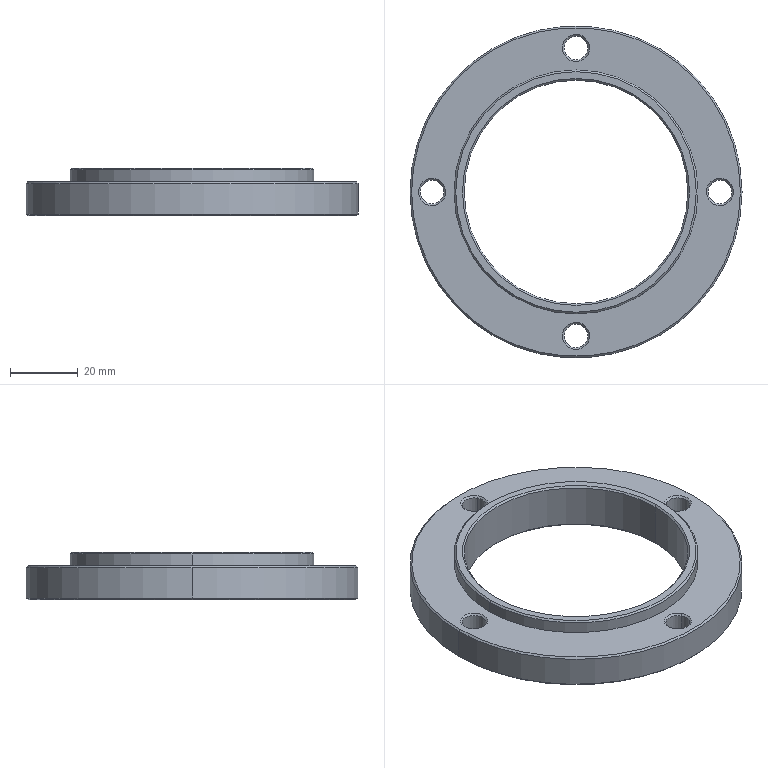Part | STEP file | 20322 | 1 solid | 43 faces | box 98 x 98 x 14 mm | volume 42100 mm3 | cone 26 | cylinder 14 | plane 3 | commonest cylinder face diameters 7 x8 66 x2 72 x2 98 x2
STEP:
#1=CARTESIAN_POINT('',(48.5,0.,10.));
#2=VERTEX_POINT('',#1);
#3=CARTESIAN_POINT('',(49.,0.,9.5));
#4=VERTEX_POINT('',#3);
#5=CARTESIAN_POINT('',(48.75,0.,9.75));
#6=DIRECTION('',(0.7071,0.,-0.7071));
#7=VECTOR('',#6,1.);
#8=LINE('',#5,#7);
#9=EDGE_CURVE('',#2,#4,#8,.T.);
#10=ORIENTED_EDGE('',*,*,#9,.T.);
#11=CARTESIAN_POINT('',(-49.,0.,9.5));
#12=VERTEX_POINT('',#11);
#13=CARTESIAN_POINT('',(0.,0.,9.5));
#14=DIRECTION('',(0.,0.,1.));
#15=AXIS2_PLACEMENT_3D('',#13,#14,$);
#16=CIRCLE('',#15,49.);
#17=EDGE_CURVE('',#4,#12,#16,.T.);
#18=ORIENTED_EDGE('',*,*,#17,.T.);
#19=CARTESIAN_POINT('',(-48.5,0.000000485,10.));
#20=VERTEX_POINT('',#19);
#21=CARTESIAN_POINT('',(-48.75,0.,9.75));
#22=DIRECTION('',(-0.7071,0.,-0.7071));
#23=VECTOR('',#22,1.);
#24=LINE('',#21,#23);
#25=EDGE_CURVE('',#20,#12,#24,.T.);
#26=ORIENTED_EDGE('',*,*,#25,.F.);
#27=CARTESIAN_POINT('',(0.,0.,10.));
#28=DIRECTION('',(0.,0.,1.));
#29=AXIS2_PLACEMENT_3D('',#27,#28,$);
#30=CIRCLE('',#29,48.5);
#31=EDGE_CURVE('',#2,#20,#30,.T.);
#32=ORIENTED_EDGE('',*,*,#31,.F.);
#33=EDGE_LOOP('',(#10,#18,#26,#32));
#34=FACE_OUTER_BOUND('',#33,.T.);
#35=CARTESIAN_POINT('',(0.,0.,58.5));
#36=DIRECTION('',(0.,0.,-1.));
#37=DIRECTION('',(1.,0.,0.));
#38=AXIS2_PLACEMENT_3D('',#35,#36,#37);
#39=CONICAL_SURFACE('',#38,0.,0.7854);
#40=ADVANCED_FACE('',(#34),#39,.T.);
#41=ORIENTED_EDGE('',*,*,#25,.T.);
#42=CARTESIAN_POINT('',(0.,0.,9.5));
#43=DIRECTION('',(0.,0.,1.));
#44=AXIS2_PLACEMENT_3D('',#42,#43,$);
#45=CIRCLE('',#44,49.);
#46=EDGE_CURVE('',#12,#4,#45,.T.);
#47=ORIENTED_EDGE('',*,*,#46,.T.);
#48=ORIENTED_EDGE('',*,*,#9,.F.);
#49=CARTESIAN_POINT('',(0.,0.,10.));
#50=DIRECTION('',(0.,0.,1.));
#51=AXIS2_PLACEMENT_3D('',#49,#50,$);
#52=CIRCLE('',#51,48.5);
#53=EDGE_CURVE('',#20,#2,#52,.T.);
#54=ORIENTED_EDGE('',*,*,#53,.F.);
#55=EDGE_LOOP('',(#41,#47,#48,#54));
#56=FACE_OUTER_BOUND('',#55,.T.);
#57=CARTESIAN_POINT('',(0.,0.,58.5));
#58=DIRECTION('',(0.,0.,-1.));
#59=DIRECTION('',(-1.,0.,0.));
#60=AXIS2_PLACEMENT_3D('',#57,#58,#59);
#61=CONICAL_SURFACE('',#60,0.,0.7854);
#62=ADVANCED_FACE('',(#56),#61,.T.);
#63=CARTESIAN_POINT('',(-49.,0.,0.5));
#64=VERTEX_POINT('',#63);
#65=CARTESIAN_POINT('',(-49.,0.,5.));
#66=DIRECTION('',(0.,0.,1.));
#67=VECTOR('',#66,1.);
#68=LINE('',#65,#67);
#69=EDGE_CURVE('',#64,#12,#68,.T.);
#70=ORIENTED_EDGE('',*,*,#69,.T.);
#71=ORIENTED_EDGE('',*,*,#17,.F.);
#72=CARTESIAN_POINT('',(49.,0.,0.5));
#73=VERTEX_POINT('',#72);
#74=CARTESIAN_POINT('',(49.,0.,5.));
#75=DIRECTION('',(0.,0.,1.));
#76=VECTOR('',#75,1.);
#77=LINE('',#74,#76);
#78=EDGE_CURVE('',#73,#4,#77,.T.);
#79=ORIENTED_EDGE('',*,*,#78,.F.);
#80=CARTESIAN_POINT('',(0.,0.,0.5));
#81=DIRECTION('',(0.,0.,1.));
#82=AXIS2_PLACEMENT_3D('',#80,#81,$);
#83=CIRCLE('',#82,49.);
#84=EDGE_CURVE('',#73,#64,#83,.T.);
#85=ORIENTED_EDGE('',*,*,#84,.T.);
#86=EDGE_LOOP('',(#70,#71,#79,#85));
#87=FACE_OUTER_BOUND('',#86,.T.);
#88=CARTESIAN_POINT('',(0.,0.,5.));
#89=DIRECTION('',(0.,0.,1.));
#90=DIRECTION('',(1.,0.,0.));
#91=AXIS2_PLACEMENT_3D('',#88,#89,#90);
#92=CYLINDRICAL_SURFACE('',#91,49.);
#93=ADVANCED_FACE('',(#87),#92,.T.);
#94=ORIENTED_EDGE('',*,*,#78,.T.);
#95=ORIENTED_EDGE('',*,*,#46,.F.);
#96=ORIENTED_EDGE('',*,*,#69,.F.);
#97=CARTESIAN_POINT('',(0.,0.,0.5));
#98=DIRECTION('',(0.,0.,1.));
#99=AXIS2_PLACEMENT_3D('',#97,#98,$);
#100=CIRCLE('',#99,49.);
#101=EDGE_CURVE('',#64,#73,#100,.T.);
#102=ORIENTED_EDGE('',*,*,#101,.T.);
#103=EDGE_LOOP('',(#94,#95,#96,#102));
#104=FACE_OUTER_BOUND('',#103,.T.);
#105=ADVANCED_FACE('',(#104),#92,.T.);
#106=CARTESIAN_POINT('',(48.5,0.,0.));
#107=VERTEX_POINT('',#106);
#108=CARTESIAN_POINT('',(48.75,0.,0.25));
#109=DIRECTION('',(0.7071,0.,0.7071));
#110=VECTOR('',#109,1.);
#111=LINE('',#108,#110);
#112=EDGE_CURVE('',#73,#107,#111,.F.);
#113=ORIENTED_EDGE('',*,*,#112,.T.);
#114=CARTESIAN_POINT('',(-48.5,0.000000092,0.));
#115=VERTEX_POINT('',#114);
#116=CARTESIAN_POINT('',(0.,0.,0.));
#117=DIRECTION('',(0.,0.,1.));
#118=AXIS2_PLACEMENT_3D('',#116,#117,$);
#119=CIRCLE('',#118,48.5);
#120=EDGE_CURVE('',#107,#115,#119,.T.);
#121=ORIENTED_EDGE('',*,*,#120,.T.);
#122=CARTESIAN_POINT('',(-48.75,0.000000092,0.25));
#123=DIRECTION('',(-0.7071,0.000000001,0.7071));
#124=VECTOR('',#123,1.);
#125=LINE('',#122,#124);
#126=EDGE_CURVE('',#64,#115,#125,.F.);
#127=ORIENTED_EDGE('',*,*,#126,.F.);
#128=ORIENTED_EDGE('',*,*,#84,.F.);
#129=EDGE_LOOP('',(#113,#121,#127,#128));
#130=FACE_OUTER_BOUND('',#129,.T.);
#131=CARTESIAN_POINT('',(0.,0.,-48.5));
#132=DIRECTION('',(0.,0.,1.));
#133=DIRECTION('',(1.,0.,0.));
#134=AXIS2_PLACEMENT_3D('',#131,#132,#133);
#135=CONICAL_SURFACE('',#134,0.,0.7854);
#136=ADVANCED_FACE('',(#130),#135,.T.);
#137=ORIENTED_EDGE('',*,*,#126,.T.);
#138=CARTESIAN_POINT('',(0.,0.,0.));
#139=DIRECTION('',(0.,0.,1.));
#140=AXIS2_PLACEMENT_3D('',#138,#139,$);
#141=CIRCLE('',#140,48.5);
#142=EDGE_CURVE('',#115,#107,#141,.T.);
#143=ORIENTED_EDGE('',*,*,#142,.T.);
#144=ORIENTED_EDGE('',*,*,#112,.F.);
#145=ORIENTED_EDGE('',*,*,#101,.F.);
#146=EDGE_LOOP('',(#137,#143,#144,#145));
#147=FACE_OUTER_BOUND('',#146,.T.);
#148=CARTESIAN_POINT('',(0.,0.,-48.5));
#149=DIRECTION('',(0.,0.,1.));
#150=DIRECTION('',(-0.9454,0.3259,0.));
#151=AXIS2_PLACEMENT_3D('',#148,#149,#150);
#152=CONICAL_SURFACE('',#151,0.,0.7854);
#153=ADVANCED_FACE('',(#147),#152,.T.);
#154=CARTESIAN_POINT('',(-33.5,-0.000000738,0.));
#155=VERTEX_POINT('',#154);
#156=CARTESIAN_POINT('',(-33.,0.,0.5));
#157=VERTEX_POINT('',#156);
#158=CARTESIAN_POINT('',(-33.25,0.,0.25));
#159=DIRECTION('',(-0.7071,0.,-0.7071));
#160=VECTOR('',#159,1.);
#161=LINE('',#158,#160);
#162=EDGE_CURVE('',#155,#157,#161,.F.);
#163=ORIENTED_EDGE('',*,*,#162,.T.);
#164=CARTESIAN_POINT('',(33.,0.,0.5));
#165=VERTEX_POINT('',#164);
#166=CARTESIAN_POINT('',(0.,0.,0.5));
#167=DIRECTION('',(0.,0.,1.));
#168=AXIS2_PLACEMENT_3D('',#166,#167,$);
#169=CIRCLE('',#168,33.);
#170=EDGE_CURVE('',#157,#165,#169,.T.);
#171=ORIENTED_EDGE('',*,*,#170,.T.);
#172=CARTESIAN_POINT('',(33.5,0.,0.));
#173=VERTEX_POINT('',#172);
#174=CARTESIAN_POINT('',(33.25,0.,0.25));
#175=DIRECTION('',(0.7071,0.,-0.7071));
#176=VECTOR('',#175,1.);
#177=LINE('',#174,#176);
#178=EDGE_CURVE('',#173,#165,#177,.F.);
#179=ORIENTED_EDGE('',*,*,#178,.F.);
#180=CARTESIAN_POINT('',(0.,0.,0.));
#181=DIRECTION('',(0.,0.,1.));
#182=AXIS2_PLACEMENT_3D('',#180,#181,$);
#183=CIRCLE('',#182,33.5);
#184=EDGE_CURVE('',#155,#173,#183,.T.);
#185=ORIENTED_EDGE('',*,*,#184,.F.);
#186=EDGE_LOOP('',(#163,#171,#179,#185));
#187=FACE_OUTER_BOUND('',#186,.T.);
#188=CARTESIAN_POINT('',(0.,0.,33.5));
#189=DIRECTION('',(0.,0.,-1.));
#190=DIRECTION('',(-0.8872,0.4614,0.));
#191=AXIS2_PLACEMENT_3D('',#188,#189,#190);
#192=CONICAL_SURFACE('',#191,0.,0.7854);
#193=ADVANCED_FACE('',(#187),#192,.F.);
#194=ORIENTED_EDGE('',*,*,#178,.T.);
#195=CARTESIAN_POINT('',(0.,0.,0.5));
#196=DIRECTION('',(0.,0.,1.));
#197=AXIS2_PLACEMENT_3D('',#195,#196,$);
#198=CIRCLE('',#197,33.);
#199=EDGE_CURVE('',#165,#157,#198,.T.);
#200=ORIENTED_EDGE('',*,*,#199,.T.);
#201=ORIENTED_EDGE('',*,*,#162,.F.);
#202=CARTESIAN_POINT('',(0.,0.,0.));
#203=DIRECTION('',(0.,0.,1.));
#204=AXIS2_PLACEMENT_3D('',#202,#203,$);
#205=CIRCLE('',#204,33.5);
#206=EDGE_CURVE('',#173,#155,#205,.T.);
#207=ORIENTED_EDGE('',*,*,#206,.F.);
#208=EDGE_LOOP('',(#194,#200,#201,#207));
#209=FACE_OUTER_BOUND('',#208,.T.);
#210=CARTESIAN_POINT('',(0.,0.,33.5));
#211=DIRECTION('',(0.,0.,-1.));
#212=DIRECTION('',(1.,0.,0.));
#213=AXIS2_PLACEMENT_3D('',#210,#211,#212);
#214=CONICAL_SURFACE('',#213,0.,0.7854);
#215=ADVANCED_FACE('',(#209),#214,.F.);
#216=ORIENTED_EDGE('',*,*,#170,.F.);
#217=CARTESIAN_POINT('',(-33.,0.,13.5));
#218=VERTEX_POINT('',#217);
#219=CARTESIAN_POINT('',(-33.,0.,5.));
#220=DIRECTION('',(0.,0.,1.));
#221=VECTOR('',#220,1.);
#222=LINE('',#219,#221);
#223=EDGE_CURVE('',#218,#157,#222,.F.);
#224=ORIENTED_EDGE('',*,*,#223,.F.);
#225=CARTESIAN_POINT('',(33.,0.,13.5));
#226=VERTEX_POINT('',#225);
#227=CARTESIAN_POINT('',(0.,0.,13.5));
#228=DIRECTION('',(0.,0.,1.));
#229=AXIS2_PLACEMENT_3D('',#227,#228,$);
#230=CIRCLE('',#229,33.);
#231=EDGE_CURVE('',#218,#226,#230,.T.);
#232=ORIENTED_EDGE('',*,*,#231,.T.);
#233=CARTESIAN_POINT('',(33.,0.,5.));
#234=DIRECTION('',(0.,0.,1.));
#235=VECTOR('',#234,1.);
#236=LINE('',#233,#235);
#237=EDGE_CURVE('',#226,#165,#236,.F.);
#238=ORIENTED_EDGE('',*,*,#237,.T.);
#239=EDGE_LOOP('',(#216,#224,#232,#238));
#240=FACE_OUTER_BOUND('',#239,.T.);
#241=CARTESIAN_POINT('',(0.,0.,5.));
#242=DIRECTION('',(0.,0.,1.));
#243=DIRECTION('',(1.,0.,0.));
#244=AXIS2_PLACEMENT_3D('',#241,#242,#243);
#245=CYLINDRICAL_SURFACE('',#244,33.);
#246=ADVANCED_FACE('',(#240),#245,.F.);
#247=ORIENTED_EDGE('',*,*,#199,.F.);
#248=ORIENTED_EDGE('',*,*,#237,.F.);
#249=CARTESIAN_POINT('',(0.,0.,13.5));
#250=DIRECTION('',(0.,0.,1.));
#251=AXIS2_PLACEMENT_3D('',#249,#250,$);
#252=CIRCLE('',#251,33.);
#253=EDGE_CURVE('',#226,#218,#252,.T.);
#254=ORIENTED_EDGE('',*,*,#253,.T.);
#255=ORIENTED_EDGE('',*,*,#223,.T.);
#256=EDGE_LOOP('',(#247,#248,#254,#255));
#257=FACE_OUTER_BOUND('',#256,.T.);
#258=ADVANCED_FACE('',(#257),#245,.F.);
#259=CARTESIAN_POINT('',(-33.5,0.000000544,14.));
#260=VERTEX_POINT('',#259);
#261=CARTESIAN_POINT('',(-33.25,0.,13.75));
#262=DIRECTION('',(-0.7071,0.,0.7071));
#263=VECTOR('',#262,1.);
#264=LINE('',#261,#263);
#265=EDGE_CURVE('',#218,#260,#264,.T.);
#266=ORIENTED_EDGE('',*,*,#265,.T.);
#267=CARTESIAN_POINT('',(33.5,0.,14.));
#268=VERTEX_POINT('',#267);
#269=CARTESIAN_POINT('',(0.,0.,14.));
#270=DIRECTION('',(0.,0.,1.));
#271=AXIS2_PLACEMENT_3D('',#269,#270,$);
#272=CIRCLE('',#271,33.5);
#273=EDGE_CURVE('',#260,#268,#272,.T.);
#274=ORIENTED_EDGE('',*,*,#273,.T.);
#275=CARTESIAN_POINT('',(33.25,0.,13.75));
#276=DIRECTION('',(0.7071,0.,0.7071));
#277=VECTOR('',#276,1.);
#278=LINE('',#275,#277);
#279=EDGE_CURVE('',#226,#268,#278,.T.);
#280=ORIENTED_EDGE('',*,*,#279,.F.);
#281=ORIENTED_EDGE('',*,*,#231,.F.);
#282=EDGE_LOOP('',(#266,#274,#280,#281));
#283=FACE_OUTER_BOUND('',#282,.T.);
#284=CARTESIAN_POINT('',(0.,0.,-19.5));
#285=DIRECTION('',(0.,0.,1.));
#286=DIRECTION('',(-0.9714,0.2374,0.));
#287=AXIS2_PLACEMENT_3D('',#284,#285,#286);
#288=CONICAL_SURFACE('',#287,0.,0.7854);
#289=ADVANCED_FACE('',(#283),#288,.F.);
#290=ORIENTED_EDGE('',*,*,#279,.T.);
#291=CARTESIAN_POINT('',(0.,0.,14.));
#292=DIRECTION('',(0.,0.,1.));
#293=AXIS2_PLACEMENT_3D('',#291,#292,$);
#294=CIRCLE('',#293,33.5);
#295=EDGE_CURVE('',#268,#260,#294,.T.);
#296=ORIENTED_EDGE('',*,*,#295,.T.);
#297=ORIENTED_EDGE('',*,*,#265,.F.);
#298=ORIENTED_EDGE('',*,*,#253,.F.);
#299=EDGE_LOOP('',(#290,#296,#297,#298));
#300=FACE_OUTER_BOUND('',#299,.T.);
#301=CARTESIAN_POINT('',(0.,0.,-19.5));
#302=DIRECTION('',(0.,0.,1.));
#303=DIRECTION('',(1.,0.,0.));
#304=AXIS2_PLACEMENT_3D('',#301,#302,#303);
#305=CONICAL_SURFACE('',#304,0.,0.7854);
#306=ADVANCED_FACE('',(#300),#305,.F.);
#307=CARTESIAN_POINT('',(35.5,0.,14.));
#308=VERTEX_POINT('',#307);
#309=CARTESIAN_POINT('',(-35.5,0.000000674,14.));
#310=VERTEX_POINT('',#309);
#311=CARTESIAN_POINT('',(0.,0.,14.));
#312=DIRECTION('',(0.,0.,1.));
#313=AXIS2_PLACEMENT_3D('',#311,#312,$);
#314=CIRCLE('',#313,35.5);
#315=EDGE_CURVE('',#308,#310,#314,.T.);
#316=ORIENTED_EDGE('',*,*,#315,.T.);
#317=CARTESIAN_POINT('',(0.,0.,14.));
#318=DIRECTION('',(0.,0.,1.));
#319=AXIS2_PLACEMENT_3D('',#317,#318,$);
#320=CIRCLE('',#319,35.5);
#321=EDGE_CURVE('',#310,#308,#320,.T.);
#322=ORIENTED_EDGE('',*,*,#321,.T.);
#323=EDGE_LOOP('',(#316,#322));
#324=FACE_OUTER_BOUND('',#323,.T.);
#325=ORIENTED_EDGE('',*,*,#273,.F.);
#326=ORIENTED_EDGE('',*,*,#295,.F.);
#327=EDGE_LOOP('',(#325,#326));
#328=FACE_BOUND('',#327,.T.);
#329=CARTESIAN_POINT('',(0.,0.,14.));
#330=DIRECTION('',(0.,0.,1.));
#331=DIRECTION('',(1.,0.,0.));
#332=AXIS2_PLACEMENT_3D('',#329,#330,#331);
#333=PLANE('',#332);
#334=ADVANCED_FACE('',(#324,#328),#333,.T.);
#335=CARTESIAN_POINT('',(36.,0.,13.5));
#336=VERTEX_POINT('',#335);
#337=CARTESIAN_POINT('',(35.75,0.,13.75));
#338=DIRECTION('',(0.7071,0.,-0.7071));
#339=VECTOR('',#338,1.);
#340=LINE('',#337,#339);
#341=EDGE_CURVE('',#308,#336,#340,.T.);
#342=ORIENTED_EDGE('',*,*,#341,.T.);
#343=CARTESIAN_POINT('',(-36.,0.,13.5));
#344=VERTEX_POINT('',#343);
#345=CARTESIAN_POINT('',(0.,0.,13.5));
#346=DIRECTION('',(0.,0.,1.));
#347=AXIS2_PLACEMENT_3D('',#345,#346,$);
#348=CIRCLE('',#347,36.);
#349=EDGE_CURVE('',#336,#344,#348,.T.);
#350=ORIENTED_EDGE('',*,*,#349,.T.);
#351=CARTESIAN_POINT('',(-35.75,0.,13.75));
#352=DIRECTION('',(-0.7071,0.,-0.7071));
#353=VECTOR('',#352,1.);
#354=LINE('',#351,#353);
#355=EDGE_CURVE('',#310,#344,#354,.T.);
#356=ORIENTED_EDGE('',*,*,#355,.F.);
#357=ORIENTED_EDGE('',*,*,#315,.F.);
#358=EDGE_LOOP('',(#342,#350,#356,#357));
#359=FACE_OUTER_BOUND('',#358,.T.);
#360=CARTESIAN_POINT('',(0.,0.,49.5));
#361=DIRECTION('',(0.,0.,-1.));
#362=DIRECTION('',(1.,0.,0.));
#363=AXIS2_PLACEMENT_3D('',#360,#361,#362);
#364=CONICAL_SURFACE('',#363,0.,0.7854);
#365=ADVANCED_FACE('',(#359),#364,.T.);
#366=ORIENTED_EDGE('',*,*,#355,.T.);
#367=CARTESIAN_POINT('',(0.,0.,13.5));
#368=DIRECTION('',(0.,0.,1.));
#369=AXIS2_PLACEMENT_3D('',#367,#368,$);
#370=CIRCLE('',#369,36.);
#371=EDGE_CURVE('',#344,#336,#370,.T.);
#372=ORIENTED_EDGE('',*,*,#371,.T.);
#373=ORIENTED_EDGE('',*,*,#341,.F.);
#374=ORIENTED_EDGE('',*,*,#321,.F.);
#375=EDGE_LOOP('',(#366,#372,#373,#374));
#376=FACE_OUTER_BOUND('',#375,.T.);
#377=CARTESIAN_POINT('',(0.,0.,49.5));
#378=DIRECTION('',(0.,0.,-1.));
#379=DIRECTION('',(-0.9522,0.3055,0.));
#380=AXIS2_PLACEMENT_3D('',#377,#378,#379);
#381=CONICAL_SURFACE('',#380,0.,0.7854);
#382=ADVANCED_FACE('',(#376),#381,.T.);
#383=CARTESIAN_POINT('',(-36.,0.,10.));
#384=VERTEX_POINT('',#383);
#385=CARTESIAN_POINT('',(-36.,0.,12.));
#386=DIRECTION('',(0.,0.,1.));
#387=VECTOR('',#386,1.);
#388=LINE('',#385,#387);
#389=EDGE_CURVE('',#384,#344,#388,.T.);
#390=ORIENTED_EDGE('',*,*,#389,.F.);
#391=CARTESIAN_POINT('',(36.,0.,10.));
#392=VERTEX_POINT('',#391);
#393=CARTESIAN_POINT('',(0.,0.,10.));
#394=DIRECTION('',(0.,0.,1.));
#395=AXIS2_PLACEMENT_3D('',#393,#394,$);
#396=CIRCLE('',#395,36.);
#397=EDGE_CURVE('',#384,#392,#396,.T.);
#398=ORIENTED_EDGE('',*,*,#397,.T.);
#399=CARTESIAN_POINT('',(36.,0.,12.));
#400=DIRECTION('',(0.,0.,1.));
#401=VECTOR('',#400,1.);
#402=LINE('',#399,#401);
#403=EDGE_CURVE('',#392,#336,#402,.T.);
#404=ORIENTED_EDGE('',*,*,#403,.T.);
#405=ORIENTED_EDGE('',*,*,#371,.F.);
#406=EDGE_LOOP('',(#390,#398,#404,#405));
#407=FACE_OUTER_BOUND('',#406,.T.);
#408=CARTESIAN_POINT('',(0.,0.,12.));
#409=DIRECTION('',(0.,0.,1.));
#410=DIRECTION('',(1.,0.,0.));
#411=AXIS2_PLACEMENT_3D('',#408,#409,#410);
#412=CYLINDRICAL_SURFACE('',#411,36.);
#413=ADVANCED_FACE('',(#407),#412,.T.);
#414=ORIENTED_EDGE('',*,*,#403,.F.);
#415=CARTESIAN_POINT('',(0.,0.,10.));
#416=DIRECTION('',(0.,0.,1.));
#417=AXIS2_PLACEMENT_3D('',#415,#416,$);
#418=CIRCLE('',#417,36.);
#419=EDGE_CURVE('',#392,#384,#418,.T.);
#420=ORIENTED_EDGE('',*,*,#419,.T.);
#421=ORIENTED_EDGE('',*,*,#389,.T.);
#422=ORIENTED_EDGE('',*,*,#349,.F.);
#423=EDGE_LOOP('',(#414,#420,#421,#422));
#424=FACE_OUTER_BOUND('',#423,.T.);
#425=ADVANCED_FACE('',(#424),#412,.T.);
#426=CARTESIAN_POINT('',(40.582,3.51,0.));
#427=VERTEX_POINT('',#426);
#428=CARTESIAN_POINT('',(40.822,3.072,0.5));
#429=VERTEX_POINT('',#428);
#430=CARTESIAN_POINT('',(40.702,3.291,0.25));
#431=DIRECTION('',(-0.339,0.6205,-0.7071));
#432=VECTOR('',#431,1.);
#433=LINE('',#430,#432);
#434=EDGE_CURVE('',#427,#429,#433,.F.);
#435=ORIENTED_EDGE('',*,*,#434,.T.);
#436=CARTESIAN_POINT('',(44.178,-3.072,0.5));
#437=VERTEX_POINT('',#436);
#438=CARTESIAN_POINT('',(42.5,0.,0.5));
#439=DIRECTION('',(0.,0.,1.));
#440=AXIS2_PLACEMENT_3D('',#438,#439,$);
#441=CIRCLE('',#440,3.5);
#442=EDGE_CURVE('',#429,#437,#441,.T.);
#443=ORIENTED_EDGE('',*,*,#442,.T.);
#444=CARTESIAN_POINT('',(44.418,-3.51,0.));
#445=VERTEX_POINT('',#444);
#446=CARTESIAN_POINT('',(44.298,-3.291,0.25));
#447=DIRECTION('',(0.339,-0.6205,-0.7071));
#448=VECTOR('',#447,1.);
#449=LINE('',#446,#448);
#450=EDGE_CURVE('',#445,#437,#449,.F.);
#451=ORIENTED_EDGE('',*,*,#450,.F.);
#452=CARTESIAN_POINT('',(42.5,0.,0.));
#453=DIRECTION('',(0.,0.,1.));
#454=AXIS2_PLACEMENT_3D('',#452,#453,$);
#455=CIRCLE('',#454,4.);
#456=EDGE_CURVE('',#427,#445,#455,.T.);
#457=ORIENTED_EDGE('',*,*,#456,.F.);
#458=EDGE_LOOP('',(#435,#443,#451,#457));
#459=FACE_OUTER_BOUND('',#458,.T.);
#460=CARTESIAN_POINT('',(42.5,0.,4.));
#461=DIRECTION('',(0.,0.,-1.));
#462=DIRECTION('',(-0.4794,0.8776,0.));
#463=AXIS2_PLACEMENT_3D('',#460,#461,#462);
#464=CONICAL_SURFACE('',#463,0.,0.7854);
#465=ADVANCED_FACE('',(#459),#464,.F.);
#466=ORIENTED_EDGE('',*,*,#450,.T.);
#467=CARTESIAN_POINT('',(42.5,0.,0.5));
#468=DIRECTION('',(0.,0.,1.));
#469=AXIS2_PLACEMENT_3D('',#467,#468,$);
#470=CIRCLE('',#469,3.5);
#471=EDGE_CURVE('',#437,#429,#470,.T.);
#472=ORIENTED_EDGE('',*,*,#471,.T.);
#473=ORIENTED_EDGE('',*,*,#434,.F.);
#474=CARTESIAN_POINT('',(42.5,0.,0.));
#475=DIRECTION('',(0.,0.,1.));
#476=AXIS2_PLACEMENT_3D('',#474,#475,$);
#477=CIRCLE('',#476,4.);
#478=EDGE_CURVE('',#445,#427,#477,.T.);
#479=ORIENTED_EDGE('',*,*,#478,.F.);
#480=EDGE_LOOP('',(#466,#472,#473,#479));
#481=FACE_OUTER_BOUND('',#480,.T.);
#482=CARTESIAN_POINT('',(42.5,0.,4.));
#483=DIRECTION('',(0.,0.,-1.));
#484=DIRECTION('',(0.4794,-0.8776,0.));
#485=AXIS2_PLACEMENT_3D('',#482,#483,#484);
#486=CONICAL_SURFACE('',#485,0.,0.7854);
#487=ADVANCED_FACE('',(#481),#486,.F.);
#488=CARTESIAN_POINT('',(40.822,3.072,9.5));
#489=VERTEX_POINT('',#488);
#490=CARTESIAN_POINT('',(44.178,-3.072,9.5));
#491=VERTEX_POINT('',#490);
#492=CARTESIAN_POINT('',(42.5,0.,9.5));
#493=DIRECTION('',(0.,0.,1.));
#494=AXIS2_PLACEMENT_3D('',#492,#493,$);
#495=CIRCLE('',#494,3.5);
#496=EDGE_CURVE('',#489,#491,#495,.T.);
#497=ORIENTED_EDGE('',*,*,#496,.T.);
#498=CARTESIAN_POINT('',(44.178,-3.072,4.845));
#499=DIRECTION('',(0.,0.,1.));
#500=VECTOR('',#499,1.);
#501=LINE('',#498,#500);
#502=EDGE_CURVE('',#491,#437,#501,.F.);
#503=ORIENTED_EDGE('',*,*,#502,.T.);
#504=ORIENTED_EDGE('',*,*,#442,.F.);
#505=CARTESIAN_POINT('',(40.822,3.072,4.845));
#506=DIRECTION('',(0.,0.,1.));
#507=VECTOR('',#506,1.);
#508=LINE('',#505,#507);
#509=EDGE_CURVE('',#489,#429,#508,.F.);
#510=ORIENTED_EDGE('',*,*,#509,.F.);
#511=EDGE_LOOP('',(#497,#503,#504,#510));
#512=FACE_OUTER_BOUND('',#511,.T.);
#513=CARTESIAN_POINT('',(42.5,0.,0.1));
#514=DIRECTION('',(0.,0.,1.));
#515=DIRECTION('',(-0.4794,0.8776,0.));
#516=AXIS2_PLACEMENT_3D('',#513,#514,#515);
#517=CYLINDRICAL_SURFACE('',#516,3.5);
#518=ADVANCED_FACE('',(#512),#517,.F.);
#519=CARTESIAN_POINT('',(42.5,0.,9.5));
#520=DIRECTION('',(0.,0.,1.));
#521=AXIS2_PLACEMENT_3D('',#519,#520,$);
#522=CIRCLE('',#521,3.5);
#523=EDGE_CURVE('',#491,#489,#522,.T.);
#524=ORIENTED_EDGE('',*,*,#523,.T.);
#525=ORIENTED_EDGE('',*,*,#509,.T.);
#526=ORIENTED_EDGE('',*,*,#471,.F.);
#527=ORIENTED_EDGE('',*,*,#502,.F.);
#528=EDGE_LOOP('',(#524,#525,#526,#527));
#529=FACE_OUTER_BOUND('',#528,.T.);
#530=ADVANCED_FACE('',(#529),#517,.F.);
#531=CARTESIAN_POINT('',(40.582,3.51,10.));
#532=VERTEX_POINT('',#531);
#533=CARTESIAN_POINT('',(40.702,3.291,9.75));
#534=DIRECTION('',(-0.339,0.6205,0.7071));
#535=VECTOR('',#534,1.);
#536=LINE('',#533,#535);
#537=EDGE_CURVE('',#489,#532,#536,.T.);
#538=ORIENTED_EDGE('',*,*,#537,.T.);
#539=CARTESIAN_POINT('',(44.418,-3.51,10.));
#540=VERTEX_POINT('',#539);
#541=CARTESIAN_POINT('',(42.5,0.,10.));
#542=DIRECTION('',(0.,0.,1.));
#543=AXIS2_PLACEMENT_3D('',#541,#542,$);
#544=CIRCLE('',#543,4.);
#545=EDGE_CURVE('',#532,#540,#544,.T.);
#546=ORIENTED_EDGE('',*,*,#545,.T.);
#547=CARTESIAN_POINT('',(44.298,-3.291,9.75));
#548=DIRECTION('',(0.339,-0.6205,0.7071));
#549=VECTOR('',#548,1.);
#550=LINE('',#547,#549);
#551=EDGE_CURVE('',#491,#540,#550,.T.);
#552=ORIENTED_EDGE('',*,*,#551,.F.);
#553=ORIENTED_EDGE('',*,*,#496,.F.);
#554=EDGE_LOOP('',(#538,#546,#552,#553));
#555=FACE_OUTER_BOUND('',#554,.T.);
#556=CARTESIAN_POINT('',(42.5,0.,6.));
#557=DIRECTION('',(0.,0.,1.));
#558=DIRECTION('',(-0.4794,0.8776,0.));
#559=AXIS2_PLACEMENT_3D('',#556,#557,#558);
#560=CONICAL_SURFACE('',#559,0.,0.7854);
#561=ADVANCED_FACE('',(#555),#560,.F.);
#562=ORIENTED_EDGE('',*,*,#551,.T.);
#563=CARTESIAN_POINT('',(42.5,0.,10.));
#564=DIRECTION('',(0.,0.,1.));
#565=AXIS2_PLACEMENT_3D('',#563,#564,$);
#566=CIRCLE('',#565,4.);
#567=EDGE_CURVE('',#540,#532,#566,.T.);
#568=ORIENTED_EDGE('',*,*,#567,.T.);
#569=ORIENTED_EDGE('',*,*,#537,.F.);
#570=ORIENTED_EDGE('',*,*,#523,.F.);
#571=EDGE_LOOP('',(#562,#568,#569,#570));
#572=FACE_OUTER_BOUND('',#571,.T.);
#573=CARTESIAN_POINT('',(42.5,0.,6.));
#574=DIRECTION('',(0.,0.,1.));
#575=DIRECTION('',(-0.128,-0.9918,0.));
#576=AXIS2_PLACEMENT_3D('',#573,#574,#575);
#577=CONICAL_SURFACE('',#576,0.,0.7854);
#578=ADVANCED_FACE('',(#572),#577,.F.);
#579=CARTESIAN_POINT('',(3.51,-40.582,0.));
#580=VERTEX_POINT('',#579);
#581=CARTESIAN_POINT('',(3.072,-40.822,0.5));
#582=VERTEX_POINT('',#581);
#583=CARTESIAN_POINT('',(3.291,-40.702,0.25));
#584=DIRECTION('',(0.6205,0.339,-0.7071));
#585=VECTOR('',#584,1.);
#586=LINE('',#583,#585);
#587=EDGE_CURVE('',#580,#582,#586,.F.);
#588=ORIENTED_EDGE('',*,*,#587,.T.);
#589=CARTESIAN_POINT('',(-3.072,-44.178,0.5));
#590=VERTEX_POINT('',#589);
#591=CARTESIAN_POINT('',(0.,-42.5,0.5));
#592=DIRECTION('',(0.,0.,1.));
#593=AXIS2_PLACEMENT_3D('',#591,#592,$);
#594=CIRCLE('',#593,3.5);
#595=EDGE_CURVE('',#582,#590,#594,.T.);
#596=ORIENTED_EDGE('',*,*,#595,.T.);
#597=CARTESIAN_POINT('',(-3.51,-44.418,0.));
#598=VERTEX_POINT('',#597);
#599=CARTESIAN_POINT('',(-3.291,-44.298,0.25));
#600=DIRECTION('',(-0.6205,-0.339,-0.7071));
#601=VECTOR('',#600,1.);
#602=LINE('',#599,#601);
#603=EDGE_CURVE('',#598,#590,#602,.F.);
#604=ORIENTED_EDGE('',*,*,#603,.F.);
#605=CARTESIAN_POINT('',(0.,-42.5,0.));
#606=DIRECTION('',(0.,0.,1.));
#607=AXIS2_PLACEMENT_3D('',#605,#606,$);
#608=CIRCLE('',#607,4.);
#609=EDGE_CURVE('',#580,#598,#608,.T.);
#610=ORIENTED_EDGE('',*,*,#609,.F.);
#611=EDGE_LOOP('',(#588,#596,#604,#610));
#612=FACE_OUTER_BOUND('',#611,.T.);
#613=CARTESIAN_POINT('',(0.,-42.5,4.));
#614=DIRECTION('',(0.,0.,-1.));
#615=DIRECTION('',(0.8776,0.4794,0.));
#616=AXIS2_PLACEMENT_3D('',#613,#614,#615);
#617=CONICAL_SURFACE('',#616,0.,0.7854);
#618=ADVANCED_FACE('',(#612),#617,.F.);
#619=ORIENTED_EDGE('',*,*,#603,.T.);
#620=CARTESIAN_POINT('',(0.,-42.5,0.5));
#621=DIRECTION('',(0.,0.,1.));
#622=AXIS2_PLACEMENT_3D('',#620,#621,$);
#623=CIRCLE('',#622,3.5);
#624=EDGE_CURVE('',#590,#582,#623,.T.);
#625=ORIENTED_EDGE('',*,*,#624,.T.);
#626=ORIENTED_EDGE('',*,*,#587,.F.);
#627=CARTESIAN_POINT('',(0.,-42.5,0.));
#628=DIRECTION('',(0.,0.,1.));
#629=AXIS2_PLACEMENT_3D('',#627,#628,$);
#630=CIRCLE('',#629,4.);
#631=EDGE_CURVE('',#598,#580,#630,.T.);
#632=ORIENTED_EDGE('',*,*,#631,.F.);
#633=EDGE_LOOP('',(#619,#625,#626,#632));
#634=FACE_OUTER_BOUND('',#633,.T.);
#635=CARTESIAN_POINT('',(0.,-42.5,4.));
#636=DIRECTION('',(0.,0.,-1.));
#637=DIRECTION('',(-0.9995,-0.03244,0.));
#638=AXIS2_PLACEMENT_3D('',#635,#636,#637);
#639=CONICAL_SURFACE('',#638,0.,0.7854);
#640=ADVANCED_FACE('',(#634),#639,.F.);
#641=CARTESIAN_POINT('',(-3.072,-44.178,9.5));
#642=VERTEX_POINT('',#641);
#643=CARTESIAN_POINT('',(3.072,-40.822,9.5));
#644=VERTEX_POINT('',#643);
#645=CARTESIAN_POINT('',(0.,-42.5,9.5));
#646=DIRECTION('',(0.,0.,1.));
#647=AXIS2_PLACEMENT_3D('',#645,#646,$);
#648=CIRCLE('',#647,3.5);
#649=EDGE_CURVE('',#642,#644,#648,.T.);
#650=ORIENTED_EDGE('',*,*,#649,.T.);
#651=CARTESIAN_POINT('',(3.072,-40.822,4.845));
#652=DIRECTION('',(0.,0.,1.));
#653=VECTOR('',#652,1.);
#654=LINE('',#651,#653);
#655=EDGE_CURVE('',#644,#582,#654,.F.);
#656=ORIENTED_EDGE('',*,*,#655,.T.);
#657=ORIENTED_EDGE('',*,*,#624,.F.);
#658=CARTESIAN_POINT('',(-3.072,-44.178,4.845));
#659=DIRECTION('',(0.,0.,1.));
#660=VECTOR('',#659,1.);
#661=LINE('',#658,#660);
#662=EDGE_CURVE('',#642,#590,#661,.F.);
#663=ORIENTED_EDGE('',*,*,#662,.F.);
#664=EDGE_LOOP('',(#650,#656,#657,#663));
#665=FACE_OUTER_BOUND('',#664,.T.);
#666=CARTESIAN_POINT('',(0.,-42.5,0.1));
#667=DIRECTION('',(0.,0.,1.));
#668=DIRECTION('',(0.8776,0.4794,0.));
#669=AXIS2_PLACEMENT_3D('',#666,#667,#668);
#670=CYLINDRICAL_SURFACE('',#669,3.5);
#671=ADVANCED_FACE('',(#665),#670,.F.);
#672=CARTESIAN_POINT('',(0.,-42.5,9.5));
#673=DIRECTION('',(0.,0.,1.));
#674=AXIS2_PLACEMENT_3D('',#672,#673,$);
#675=CIRCLE('',#674,3.5);
#676=EDGE_CURVE('',#644,#642,#675,.T.);
#677=ORIENTED_EDGE('',*,*,#676,.T.);
#678=ORIENTED_EDGE('',*,*,#662,.T.);
#679=ORIENTED_EDGE('',*,*,#595,.F.);
#680=ORIENTED_EDGE('',*,*,#655,.F.);
#681=EDGE_LOOP('',(#677,#678,#679,#680));
#682=FACE_OUTER_BOUND('',#681,.T.);
#683=ADVANCED_FACE('',(#682),#670,.F.);
#684=CARTESIAN_POINT('',(3.51,-40.582,10.));
#685=VERTEX_POINT('',#684);
#686=CARTESIAN_POINT('',(3.291,-40.702,9.75));
#687=DIRECTION('',(0.6205,0.339,0.7071));
#688=VECTOR('',#687,1.);
#689=LINE('',#686,#688);
#690=EDGE_CURVE('',#644,#685,#689,.T.);
#691=ORIENTED_EDGE('',*,*,#690,.T.);
#692=CARTESIAN_POINT('',(-3.51,-44.418,10.));
#693=VERTEX_POINT('',#692);
#694=CARTESIAN_POINT('',(0.,-42.5,10.));
#695=DIRECTION('',(0.,0.,1.));
#696=AXIS2_PLACEMENT_3D('',#694,#695,$);
#697=CIRCLE('',#696,4.);
#698=EDGE_CURVE('',#685,#693,#697,.T.);
#699=ORIENTED_EDGE('',*,*,#698,.T.);
#700=CARTESIAN_POINT('',(-3.291,-44.298,9.75));
#701=DIRECTION('',(-0.6205,-0.339,0.7071));
#702=VECTOR('',#701,1.);
#703=LINE('',#700,#702);
#704=EDGE_CURVE('',#642,#693,#703,.T.);
#705=ORIENTED_EDGE('',*,*,#704,.F.);
#706=ORIENTED_EDGE('',*,*,#676,.F.);
#707=EDGE_LOOP('',(#691,#699,#705,#706));
#708=FACE_OUTER_BOUND('',#707,.T.);
#709=CARTESIAN_POINT('',(0.,-42.5,6.));
#710=DIRECTION('',(0.,0.,1.));
#711=DIRECTION('',(0.8776,0.4794,0.));
#712=AXIS2_PLACEMENT_3D('',#709,#710,#711);
#713=CONICAL_SURFACE('',#712,0.,0.7854);
#714=ADVANCED_FACE('',(#708),#713,.F.);
#715=ORIENTED_EDGE('',*,*,#704,.T.);
#716=CARTESIAN_POINT('',(0.,-42.5,10.));
#717=DIRECTION('',(0.,0.,1.));
#718=AXIS2_PLACEMENT_3D('',#716,#717,$);
#719=CIRCLE('',#718,4.);
#720=EDGE_CURVE('',#693,#685,#719,.T.);
#721=ORIENTED_EDGE('',*,*,#720,.T.);
#722=ORIENTED_EDGE('',*,*,#690,.F.);
#723=ORIENTED_EDGE('',*,*,#649,.F.);
#724=EDGE_LOOP('',(#715,#721,#722,#723));
#725=FACE_OUTER_BOUND('',#724,.T.);
#726=CARTESIAN_POINT('',(0.,-42.5,6.));
#727=DIRECTION('',(0.,0.,1.));
#728=DIRECTION('',(-0.9918,0.128,0.));
#729=AXIS2_PLACEMENT_3D('',#726,#727,#728);
#730=CONICAL_SURFACE('',#729,0.,0.7854);
#731=ADVANCED_FACE('',(#725),#730,.F.);
#732=CARTESIAN_POINT('',(-44.418,3.51,0.));
#733=VERTEX_POINT('',#732);
#734=CARTESIAN_POINT('',(-44.178,3.072,0.5));
#735=VERTEX_POINT('',#734);
#736=CARTESIAN_POINT('',(-44.298,3.291,0.25));
#737=DIRECTION('',(-0.339,0.6205,-0.7071));
#738=VECTOR('',#737,1.);
#739=LINE('',#736,#738);
#740=EDGE_CURVE('',#733,#735,#739,.F.);
#741=ORIENTED_EDGE('',*,*,#740,.T.);
#742=CARTESIAN_POINT('',(-40.822,-3.072,0.5));
#743=VERTEX_POINT('',#742);
#744=CARTESIAN_POINT('',(-42.5,0.,0.5));
#745=DIRECTION('',(0.,0.,1.));
#746=AXIS2_PLACEMENT_3D('',#744,#745,$);
#747=CIRCLE('',#746,3.5);
#748=EDGE_CURVE('',#735,#743,#747,.T.);
#749=ORIENTED_EDGE('',*,*,#748,.T.);
#750=CARTESIAN_POINT('',(-40.582,-3.51,0.));
#751=VERTEX_POINT('',#750);
#752=CARTESIAN_POINT('',(-40.702,-3.291,0.25));
#753=DIRECTION('',(0.339,-0.6205,-0.7071));
#754=VECTOR('',#753,1.);
#755=LINE('',#752,#754);
#756=EDGE_CURVE('',#751,#743,#755,.F.);
#757=ORIENTED_EDGE('',*,*,#756,.F.);
#758=CARTESIAN_POINT('',(-42.5,0.,0.));
#759=DIRECTION('',(0.,0.,1.));
#760=AXIS2_PLACEMENT_3D('',#758,#759,$);
#761=CIRCLE('',#760,4.);
#762=EDGE_CURVE('',#733,#751,#761,.T.);
#763=ORIENTED_EDGE('',*,*,#762,.F.);
#764=EDGE_LOOP('',(#741,#749,#757,#763));
#765=FACE_OUTER_BOUND('',#764,.T.);
#766=CARTESIAN_POINT('',(-42.5,0.,4.));
#767=DIRECTION('',(0.,0.,-1.));
#768=DIRECTION('',(-0.4178,0.9085,0.));
#769=AXIS2_PLACEMENT_3D('',#766,#767,#768);
#770=CONICAL_SURFACE('',#769,0.,0.7854);
#771=ADVANCED_FACE('',(#765),#770,.F.);
#772=ORIENTED_EDGE('',*,*,#756,.T.);
#773=CARTESIAN_POINT('',(-42.5,0.,0.5));
#774=DIRECTION('',(0.,0.,1.));
#775=AXIS2_PLACEMENT_3D('',#773,#774,$);
#776=CIRCLE('',#775,3.5);
#777=EDGE_CURVE('',#743,#735,#776,.T.);
#778=ORIENTED_EDGE('',*,*,#777,.T.);
#779=ORIENTED_EDGE('',*,*,#740,.F.);
#780=CARTESIAN_POINT('',(-42.5,0.,0.));
#781=DIRECTION('',(0.,0.,1.));
#782=AXIS2_PLACEMENT_3D('',#780,#781,$);
#783=CIRCLE('',#782,4.);
#784=EDGE_CURVE('',#751,#733,#783,.T.);
#785=ORIENTED_EDGE('',*,*,#784,.F.);
#786=EDGE_LOOP('',(#772,#778,#779,#785));
#787=FACE_OUTER_BOUND('',#786,.T.);
#788=CARTESIAN_POINT('',(-42.5,0.,4.));
#789=DIRECTION('',(0.,0.,-1.));
#790=DIRECTION('',(0.4794,-0.8776,0.));
#791=AXIS2_PLACEMENT_3D('',#788,#789,#790);
#792=CONICAL_SURFACE('',#791,0.,0.7854);
#793=ADVANCED_FACE('',(#787),#792,.F.);
#794=CARTESIAN_POINT('',(-40.822,-3.072,9.5));
#795=VERTEX_POINT('',#794);
#796=CARTESIAN_POINT('',(-44.178,3.072,9.5));
#797=VERTEX_POINT('',#796);
#798=CARTESIAN_POINT('',(-42.5,0.,9.5));
#799=DIRECTION('',(0.,0.,1.));
#800=AXIS2_PLACEMENT_3D('',#798,#799,$);
#801=CIRCLE('',#800,3.5);
#802=EDGE_CURVE('',#795,#797,#801,.T.);
#803=ORIENTED_EDGE('',*,*,#802,.T.);
#804=CARTESIAN_POINT('',(-44.178,3.072,4.845));
#805=DIRECTION('',(0.,0.,1.));
#806=VECTOR('',#805,1.);
#807=LINE('',#804,#806);
#808=EDGE_CURVE('',#797,#735,#807,.F.);
#809=ORIENTED_EDGE('',*,*,#808,.T.);
#810=ORIENTED_EDGE('',*,*,#777,.F.);
#811=CARTESIAN_POINT('',(-40.822,-3.072,4.845));
#812=DIRECTION('',(0.,0.,1.));
#813=VECTOR('',#812,1.);
#814=LINE('',#811,#813);
#815=EDGE_CURVE('',#795,#743,#814,.F.);
#816=ORIENTED_EDGE('',*,*,#815,.F.);
#817=EDGE_LOOP('',(#803,#809,#810,#816));
#818=FACE_OUTER_BOUND('',#817,.T.);
#819=CARTESIAN_POINT('',(-42.5,0.,0.1));
#820=DIRECTION('',(0.,0.,1.));
#821=DIRECTION('',(0.4794,-0.8776,0.));
#822=AXIS2_PLACEMENT_3D('',#819,#820,#821);
#823=CYLINDRICAL_SURFACE('',#822,3.5);
#824=ADVANCED_FACE('',(#818),#823,.F.);
#825=CARTESIAN_POINT('',(-42.5,0.,9.5));
#826=DIRECTION('',(0.,0.,1.));
#827=AXIS2_PLACEMENT_3D('',#825,#826,$);
#828=CIRCLE('',#827,3.5);
#829=EDGE_CURVE('',#797,#795,#828,.T.);
#830=ORIENTED_EDGE('',*,*,#829,.T.);
#831=ORIENTED_EDGE('',*,*,#815,.T.);
#832=ORIENTED_EDGE('',*,*,#748,.F.);
#833=ORIENTED_EDGE('',*,*,#808,.F.);
#834=EDGE_LOOP('',(#830,#831,#832,#833));
#835=FACE_OUTER_BOUND('',#834,.T.);
#836=ADVANCED_FACE('',(#835),#823,.F.);
#837=CARTESIAN_POINT('',(-44.418,3.51,10.));
#838=VERTEX_POINT('',#837);
#839=CARTESIAN_POINT('',(-44.298,3.291,9.75));
#840=DIRECTION('',(-0.339,0.6205,0.7071));
#841=VECTOR('',#840,1.);
#842=LINE('',#839,#841);
#843=EDGE_CURVE('',#797,#838,#842,.T.);
#844=ORIENTED_EDGE('',*,*,#843,.T.);
#845=CARTESIAN_POINT('',(-40.582,-3.51,10.));
#846=VERTEX_POINT('',#845);
#847=CARTESIAN_POINT('',(-42.5,0.,10.));
#848=DIRECTION('',(0.,0.,1.));
#849=AXIS2_PLACEMENT_3D('',#847,#848,$);
#850=CIRCLE('',#849,4.);
#851=EDGE_CURVE('',#838,#846,#850,.T.);
#852=ORIENTED_EDGE('',*,*,#851,.T.);
#853=CARTESIAN_POINT('',(-40.702,-3.291,9.75));
#854=DIRECTION('',(0.339,-0.6205,0.7071));
#855=VECTOR('',#854,1.);
#856=LINE('',#853,#855);
#857=EDGE_CURVE('',#795,#846,#856,.T.);
#858=ORIENTED_EDGE('',*,*,#857,.F.);
#859=ORIENTED_EDGE('',*,*,#829,.F.);
#860=EDGE_LOOP('',(#844,#852,#858,#859));
#861=FACE_OUTER_BOUND('',#860,.T.);
#862=CARTESIAN_POINT('',(-42.5,0.,6.));
#863=DIRECTION('',(0.,0.,1.));
#864=DIRECTION('',(-0.4178,0.9085,0.));
#865=AXIS2_PLACEMENT_3D('',#862,#863,#864);
#866=CONICAL_SURFACE('',#865,0.,0.7854);
#867=ADVANCED_FACE('',(#861),#866,.F.);
#868=ORIENTED_EDGE('',*,*,#857,.T.);
#869=CARTESIAN_POINT('',(-42.5,0.,10.));
#870=DIRECTION('',(0.,0.,1.));
#871=AXIS2_PLACEMENT_3D('',#869,#870,$);
#872=CIRCLE('',#871,4.);
#873=EDGE_CURVE('',#846,#838,#872,.T.);
#874=ORIENTED_EDGE('',*,*,#873,.T.);
#875=ORIENTED_EDGE('',*,*,#843,.F.);
#876=ORIENTED_EDGE('',*,*,#802,.F.);
#877=EDGE_LOOP('',(#868,#874,#875,#876));
#878=FACE_OUTER_BOUND('',#877,.T.);
#879=CARTESIAN_POINT('',(-42.5,0.,6.));
#880=DIRECTION('',(0.,0.,1.));
#881=DIRECTION('',(0.4794,-0.8776,0.));
#882=AXIS2_PLACEMENT_3D('',#879,#880,#881);
#883=CONICAL_SURFACE('',#882,0.,0.7854);
#884=ADVANCED_FACE('',(#878),#883,.F.);
#885=ORIENTED_EDGE('',*,*,#31,.T.);
#886=ORIENTED_EDGE('',*,*,#53,.T.);
#887=EDGE_LOOP('',(#885,#886));
#888=FACE_OUTER_BOUND('',#887,.T.);
#889=CARTESIAN_POINT('',(3.51,44.418,10.));
#890=VERTEX_POINT('',#889);
#891=CARTESIAN_POINT('',(-3.51,40.582,10.));
#892=VERTEX_POINT('',#891);
#893=CARTESIAN_POINT('',(0.,42.5,10.));
#894=DIRECTION('',(0.,0.,1.));
#895=AXIS2_PLACEMENT_3D('',#893,#894,$);
#896=CIRCLE('',#895,4.);
#897=EDGE_CURVE('',#890,#892,#896,.T.);
#898=ORIENTED_EDGE('',*,*,#897,.F.);
#899=CARTESIAN_POINT('',(0.,42.5,10.));
#900=DIRECTION('',(0.,0.,1.));
#901=AXIS2_PLACEMENT_3D('',#899,#900,$);
#902=CIRCLE('',#901,4.);
#903=EDGE_CURVE('',#892,#890,#902,.T.);
#904=ORIENTED_EDGE('',*,*,#903,.F.);
#905=EDGE_LOOP('',(#898,#904));
#906=FACE_BOUND('',#905,.T.);
#907=ORIENTED_EDGE('',*,*,#873,.F.);
#908=ORIENTED_EDGE('',*,*,#851,.F.);
#909=EDGE_LOOP('',(#907,#908));
#910=FACE_BOUND('',#909,.T.);
#911=ORIENTED_EDGE('',*,*,#720,.F.);
#912=ORIENTED_EDGE('',*,*,#698,.F.);
#913=EDGE_LOOP('',(#911,#912));
#914=FACE_BOUND('',#913,.T.);
#915=ORIENTED_EDGE('',*,*,#567,.F.);
#916=ORIENTED_EDGE('',*,*,#545,.F.);
#917=EDGE_LOOP('',(#915,#916));
#918=FACE_BOUND('',#917,.T.);
#919=ORIENTED_EDGE('',*,*,#419,.F.);
#920=ORIENTED_EDGE('',*,*,#397,.F.);
#921=EDGE_LOOP('',(#919,#920));
#922=FACE_BOUND('',#921,.T.);
#923=CARTESIAN_POINT('',(0.,0.,10.));
#924=DIRECTION('',(0.,0.,1.));
#925=DIRECTION('',(1.,0.,0.));
#926=AXIS2_PLACEMENT_3D('',#923,#924,#925);
#927=PLANE('',#926);
#928=ADVANCED_FACE('',(#888,#906,#910,#914,#918,#922),#927,.T.);
#929=CARTESIAN_POINT('',(-3.072,40.822,9.5));
#930=VERTEX_POINT('',#929);
#931=CARTESIAN_POINT('',(-3.291,40.702,9.75));
#932=DIRECTION('',(-0.6205,-0.339,0.7071));
#933=VECTOR('',#932,1.);
#934=LINE('',#931,#933);
#935=EDGE_CURVE('',#930,#892,#934,.T.);
#936=ORIENTED_EDGE('',*,*,#935,.T.);
#937=ORIENTED_EDGE('',*,*,#903,.T.);
#938=CARTESIAN_POINT('',(3.072,44.178,9.5));
#939=VERTEX_POINT('',#938);
#940=CARTESIAN_POINT('',(3.291,44.298,9.75));
#941=DIRECTION('',(0.6205,0.339,0.7071));
#942=VECTOR('',#941,1.);
#943=LINE('',#940,#942);
#944=EDGE_CURVE('',#939,#890,#943,.T.);
#945=ORIENTED_EDGE('',*,*,#944,.F.);
#946=CARTESIAN_POINT('',(0.,42.5,9.5));
#947=DIRECTION('',(0.,0.,1.));
#948=AXIS2_PLACEMENT_3D('',#946,#947,$);
#949=CIRCLE('',#948,3.5);
#950=EDGE_CURVE('',#930,#939,#949,.T.);
#951=ORIENTED_EDGE('',*,*,#950,.F.);
#952=EDGE_LOOP('',(#936,#937,#945,#951));
#953=FACE_OUTER_BOUND('',#952,.T.);
#954=CARTESIAN_POINT('',(0.,42.5,6.));
#955=DIRECTION('',(0.,0.,1.));
#956=DIRECTION('',(-0.8776,-0.4794,0.));
#957=AXIS2_PLACEMENT_3D('',#954,#955,#956);
#958=CONICAL_SURFACE('',#957,0.,0.7854);
#959=ADVANCED_FACE('',(#953),#958,.F.);
#960=ORIENTED_EDGE('',*,*,#944,.T.);
#961=ORIENTED_EDGE('',*,*,#897,.T.);
#962=ORIENTED_EDGE('',*,*,#935,.F.);
#963=CARTESIAN_POINT('',(0.,42.5,9.5));
#964=DIRECTION('',(0.,0.,1.));
#965=AXIS2_PLACEMENT_3D('',#963,#964,$);
#966=CIRCLE('',#965,3.5);
#967=EDGE_CURVE('',#939,#930,#966,.T.);
#968=ORIENTED_EDGE('',*,*,#967,.F.);
#969=EDGE_LOOP('',(#960,#961,#962,#968));
#970=FACE_OUTER_BOUND('',#969,.T.);
#971=CARTESIAN_POINT('',(0.,42.5,6.));
#972=DIRECTION('',(0.,0.,1.));
#973=DIRECTION('',(0.9995,0.03244,0.));
#974=AXIS2_PLACEMENT_3D('',#971,#972,#973);
#975=CONICAL_SURFACE('',#974,0.,0.7854);
#976=ADVANCED_FACE('',(#970),#975,.F.);
#977=ORIENTED_EDGE('',*,*,#142,.F.);
#978=ORIENTED_EDGE('',*,*,#120,.F.);
#979=EDGE_LOOP('',(#977,#978));
#980=FACE_OUTER_BOUND('',#979,.T.);
#981=CARTESIAN_POINT('',(-3.51,40.582,0.));
#982=VERTEX_POINT('',#981);
#983=CARTESIAN_POINT('',(3.51,44.418,0.));
#984=VERTEX_POINT('',#983);
#985=CARTESIAN_POINT('',(0.,42.5,0.));
#986=DIRECTION('',(0.,0.,1.));
#987=AXIS2_PLACEMENT_3D('',#985,#986,$);
#988=CIRCLE('',#987,4.);
#989=EDGE_CURVE('',#982,#984,#988,.T.);
#990=ORIENTED_EDGE('',*,*,#989,.T.);
#991=CARTESIAN_POINT('',(0.,42.5,0.));
#992=DIRECTION('',(0.,0.,1.));
#993=AXIS2_PLACEMENT_3D('',#991,#992,$);
#994=CIRCLE('',#993,4.);
#995=EDGE_CURVE('',#984,#982,#994,.T.);
#996=ORIENTED_EDGE('',*,*,#995,.T.);
#997=EDGE_LOOP('',(#990,#996));
#998=FACE_BOUND('',#997,.T.);
#999=ORIENTED_EDGE('',*,*,#762,.T.);
#1000=ORIENTED_EDGE('',*,*,#784,.T.);
#1001=EDGE_LOOP('',(#999,#1000));
#1002=FACE_BOUND('',#1001,.T.);
#1003=ORIENTED_EDGE('',*,*,#609,.T.);
#1004=ORIENTED_EDGE('',*,*,#631,.T.);
#1005=EDGE_LOOP('',(#1003,#1004));
#1006=FACE_BOUND('',#1005,.T.);
#1007=ORIENTED_EDGE('',*,*,#456,.T.);
#1008=ORIENTED_EDGE('',*,*,#478,.T.);
#1009=EDGE_LOOP('',(#1007,#1008));
#1010=FACE_BOUND('',#1009,.T.);
#1011=ORIENTED_EDGE('',*,*,#206,.T.);
#1012=ORIENTED_EDGE('',*,*,#184,.T.);
#1013=EDGE_LOOP('',(#1011,#1012));
#1014=FACE_BOUND('',#1013,.T.);
#1015=CARTESIAN_POINT('',(0.,0.,0.));
#1016=DIRECTION('',(0.,0.,1.));
#1017=DIRECTION('',(1.,0.,0.));
#1018=AXIS2_PLACEMENT_3D('',#1015,#1016,#1017);
#1019=PLANE('',#1018);
#1020=ADVANCED_FACE('',(#980,#998,#1002,#1006,#1010,#1014),#1019,.F.);
#1021=CARTESIAN_POINT('',(-3.072,40.822,0.5));
#1022=VERTEX_POINT('',#1021);
#1023=CARTESIAN_POINT('',(3.072,44.178,0.5));
#1024=VERTEX_POINT('',#1023);
#1025=CARTESIAN_POINT('',(0.,42.5,0.5));
#1026=DIRECTION('',(0.,0.,1.));
#1027=AXIS2_PLACEMENT_3D('',#1025,#1026,$);
#1028=CIRCLE('',#1027,3.5);
#1029=EDGE_CURVE('',#1022,#1024,#1028,.T.);
#1030=ORIENTED_EDGE('',*,*,#1029,.F.);
#1031=CARTESIAN_POINT('',(-3.072,40.822,4.845));
#1032=DIRECTION('',(0.,0.,1.));
#1033=VECTOR('',#1032,1.);
#1034=LINE('',#1031,#1033);
#1035=EDGE_CURVE('',#930,#1022,#1034,.F.);
#1036=ORIENTED_EDGE('',*,*,#1035,.F.);
#1037=ORIENTED_EDGE('',*,*,#950,.T.);
#1038=CARTESIAN_POINT('',(3.072,44.178,4.845));
#1039=DIRECTION('',(0.,0.,1.));
#1040=VECTOR('',#1039,1.);
#1041=LINE('',#1038,#1040);
#1042=EDGE_CURVE('',#939,#1024,#1041,.F.);
#1043=ORIENTED_EDGE('',*,*,#1042,.T.);
#1044=EDGE_LOOP('',(#1030,#1036,#1037,#1043));
#1045=FACE_OUTER_BOUND('',#1044,.T.);
#1046=CARTESIAN_POINT('',(0.,42.5,0.1));
#1047=DIRECTION('',(0.,0.,1.));
#1048=DIRECTION('',(-0.8776,-0.4794,0.));
#1049=AXIS2_PLACEMENT_3D('',#1046,#1047,#1048);
#1050=CYLINDRICAL_SURFACE('',#1049,3.5);
#1051=ADVANCED_FACE('',(#1045),#1050,.F.);
#1052=CARTESIAN_POINT('',(0.,42.5,0.5));
#1053=DIRECTION('',(0.,0.,1.));
#1054=AXIS2_PLACEMENT_3D('',#1052,#1053,$);
#1055=CIRCLE('',#1054,3.5);
#1056=EDGE_CURVE('',#1024,#1022,#1055,.T.);
#1057=ORIENTED_EDGE('',*,*,#1056,.F.);
#1058=ORIENTED_EDGE('',*,*,#1042,.F.);
#1059=ORIENTED_EDGE('',*,*,#967,.T.);
#1060=ORIENTED_EDGE('',*,*,#1035,.T.);
#1061=EDGE_LOOP('',(#1057,#1058,#1059,#1060));
#1062=FACE_OUTER_BOUND('',#1061,.T.);
#1063=ADVANCED_FACE('',(#1062),#1050,.F.);
#1064=CARTESIAN_POINT('',(-3.291,40.702,0.25));
#1065=DIRECTION('',(-0.6205,-0.339,-0.7071));
#1066=VECTOR('',#1065,1.);
#1067=LINE('',#1064,#1066);
#1068=EDGE_CURVE('',#982,#1022,#1067,.F.);
#1069=ORIENTED_EDGE('',*,*,#1068,.T.);
#1070=ORIENTED_EDGE('',*,*,#1029,.T.);
#1071=CARTESIAN_POINT('',(3.291,44.298,0.25));
#1072=DIRECTION('',(0.6205,0.339,-0.7071));
#1073=VECTOR('',#1072,1.);
#1074=LINE('',#1071,#1073);
#1075=EDGE_CURVE('',#984,#1024,#1074,.F.);
#1076=ORIENTED_EDGE('',*,*,#1075,.F.);
#1077=ORIENTED_EDGE('',*,*,#989,.F.);
#1078=EDGE_LOOP('',(#1069,#1070,#1076,#1077));
#1079=FACE_OUTER_BOUND('',#1078,.T.);
#1080=CARTESIAN_POINT('',(0.,42.5,4.));
#1081=DIRECTION('',(0.,0.,-1.));
#1082=DIRECTION('',(-0.8776,-0.4794,0.));
#1083=AXIS2_PLACEMENT_3D('',#1080,#1081,#1082);
#1084=CONICAL_SURFACE('',#1083,0.,0.7854);
#1085=ADVANCED_FACE('',(#1079),#1084,.F.);
#1086=ORIENTED_EDGE('',*,*,#1075,.T.);
#1087=ORIENTED_EDGE('',*,*,#1056,.T.);
#1088=ORIENTED_EDGE('',*,*,#1068,.F.);
#1089=ORIENTED_EDGE('',*,*,#995,.F.);
#1090=EDGE_LOOP('',(#1086,#1087,#1088,#1089));
#1091=FACE_OUTER_BOUND('',#1090,.T.);
#1092=CARTESIAN_POINT('',(0.,42.5,4.));
#1093=DIRECTION('',(0.,0.,-1.));
#1094=DIRECTION('',(0.8776,0.4794,0.));
#1095=AXIS2_PLACEMENT_3D('',#1092,#1093,#1094);
#1096=CONICAL_SURFACE('',#1095,0.,0.7854);
#1097=ADVANCED_FACE('',(#1091),#1096,.F.);
#1098=CLOSED_SHELL('',(#40,#62,#93,#105,#136,#153,#193,#215,#246,#258,#289,#306,#334,#365,#382,#413,#425,#465,#487,#518,#530,#561,#578,#618,#640,#671,#683,#714,#731,#771,#793,#824,#836,#867,#884,#928,#959,#976,#1020,#1051,#1063,#1085,#1097));
#1099=MANIFOLD_SOLID_BREP('',#1098);
#1100=(LENGTH_UNIT()NAMED_UNIT(*)SI_UNIT(.MILLI.,.METRE.));
#1101=UNCERTAINTY_MEASURE_WITH_UNIT(LENGTH_MEASURE(0.005),#1100,'','');
#1102=(NAMED_UNIT(*)PLANE_ANGLE_UNIT()SI_UNIT($,.RADIAN.));
#1103=(NAMED_UNIT(*)SI_UNIT($,.STERADIAN.)SOLID_ANGLE_UNIT());
#1104=(GEOMETRIC_REPRESENTATION_CONTEXT(3)GLOBAL_UNCERTAINTY_ASSIGNED_CONTEXT((#1101))GLOBAL_UNIT_ASSIGNED_CONTEXT((#1100,#1102,#1103))REPRESENTATION_CONTEXT('',''));
#1105=ADVANCED_BREP_SHAPE_REPRESENTATION('',(#1099),#1104);